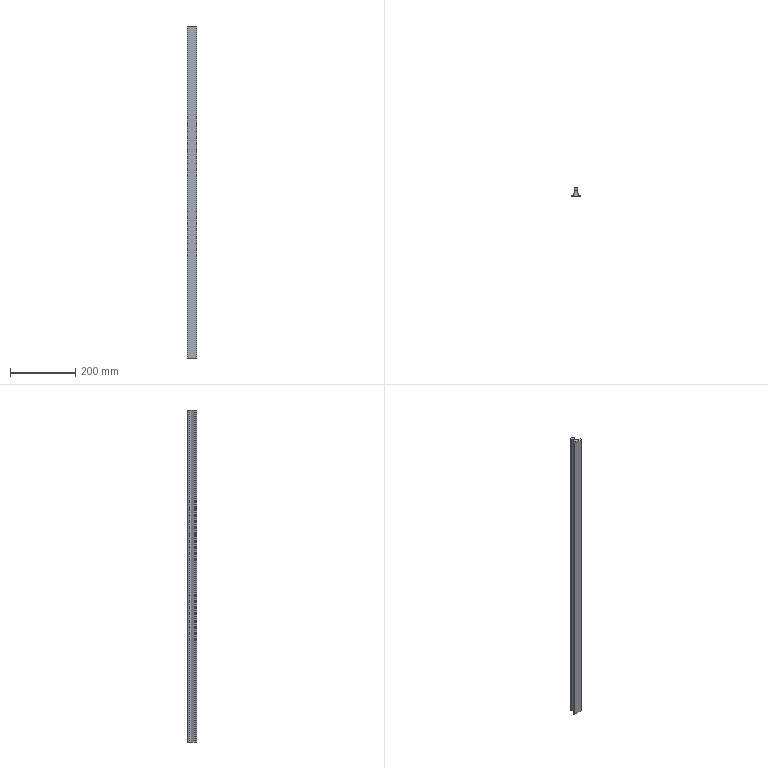Part | STEP file | SBR16S round rail_default<machined> | 2 solids | 16 faces | box 30 x 28.5 x 1020 mm | volume 387317 mm3 | plane 13 | cylinder 3 | commonest cylinder face diameters 12 x3
STEP:
#1=CARTESIAN_POINT('',(0.,0.,0.));
#2=DIRECTION('',(0.,0.,1.));
#3=DIRECTION('',(1.,0.,0.));
#4=AXIS2_PLACEMENT_3D('',#1,#2,#3);
#5=CARTESIAN_POINT('',(6.,0.,1020.));
#6=VERTEX_POINT('',#5);
#7=CARTESIAN_POINT('',(-6.,0.,1020.));
#8=VERTEX_POINT('',#7);
#9=CARTESIAN_POINT('',(0.,0.,1020.));
#10=DIRECTION('',(0.,0.,1.));
#11=DIRECTION('',(1.,0.,0.));
#12=AXIS2_PLACEMENT_3D('',#9,#10,#11);
#13=CIRCLE('',#12,6.);
#14=CARTESIAN_POINT('',(0.,0.,1020.));
#15=DIRECTION('',(0.,0.,-1.));
#16=DIRECTION('',(-1.,0.,0.));
#17=AXIS2_PLACEMENT_3D('',#14,#15,#16);
#18=CYLINDRICAL_SURFACE('',#17,6.);
#19=CARTESIAN_POINT('',(3.142,0.));
#20=DIRECTION('',(-1.,0.));
#21=VECTOR('',#20,1.);
#22=LINE('',#19,#21);
#23=(GEOMETRIC_REPRESENTATION_CONTEXT(2)PARAMETRIC_REPRESENTATION_CONTEXT()REPRESENTATION_CONTEXT('',''));
#24=DEFINITIONAL_REPRESENTATION('',(#22),#23);
#25=PCURVE('',#18,#24);
#26=CARTESIAN_POINT('',(0.,0.,1020.));
#27=DIRECTION('',(0.,0.,1.));
#28=DIRECTION('',(1.,0.,0.));
#29=AXIS2_PLACEMENT_3D('',#26,#27,#28);
#30=PLANE('',#29);
#31=CARTESIAN_POINT('',(0.,0.));
#32=DIRECTION('',(1.,0.));
#33=AXIS2_PLACEMENT_2D('',#31,#32);
#34=CIRCLE('',#33,6.);
#35=(GEOMETRIC_REPRESENTATION_CONTEXT(2)PARAMETRIC_REPRESENTATION_CONTEXT()REPRESENTATION_CONTEXT('',''));
#36=DEFINITIONAL_REPRESENTATION('',(#34),#35);
#37=PCURVE('',#30,#36);
#38=SURFACE_CURVE('',#13,(#25,#37),.PCURVE_S1.);
#39=EDGE_CURVE('',#6,#8,#38,.T.);
#40=ORIENTED_EDGE('',*,*,#39,.F.);
#41=CARTESIAN_POINT('',(6.,0.,0.));
#42=VERTEX_POINT('',#41);
#43=CARTESIAN_POINT('',(6.,0.,1020.));
#44=DIRECTION('',(0.,0.,-1.));
#45=VECTOR('',#44,1.);
#46=LINE('',#43,#45);
#47=CARTESIAN_POINT('',(3.142,0.));
#48=DIRECTION('',(0.,1.));
#49=VECTOR('',#48,1.);
#50=LINE('',#47,#49);
#51=(GEOMETRIC_REPRESENTATION_CONTEXT(2)PARAMETRIC_REPRESENTATION_CONTEXT()REPRESENTATION_CONTEXT('',''));
#52=DEFINITIONAL_REPRESENTATION('',(#50),#51);
#53=PCURVE('',#18,#52);
#54=CARTESIAN_POINT('',(0.,0.,1020.));
#55=DIRECTION('',(0.,0.,-1.));
#56=DIRECTION('',(-1.,0.,0.));
#57=AXIS2_PLACEMENT_3D('',#54,#55,#56);
#58=CYLINDRICAL_SURFACE('',#57,6.);
#59=CARTESIAN_POINT('',(3.142,0.));
#60=DIRECTION('',(0.,1.));
#61=VECTOR('',#60,1.);
#62=LINE('',#59,#61);
#63=(GEOMETRIC_REPRESENTATION_CONTEXT(2)PARAMETRIC_REPRESENTATION_CONTEXT()REPRESENTATION_CONTEXT('',''));
#64=DEFINITIONAL_REPRESENTATION('',(#62),#63);
#65=PCURVE('',#58,#64);
#66=SURFACE_CURVE('',#46,(#53,#65),.PCURVE_S1.);
#67=EDGE_CURVE('',#6,#42,#66,.T.);
#68=ORIENTED_EDGE('',*,*,#67,.T.);
#69=CARTESIAN_POINT('',(-6.,0.,0.));
#70=VERTEX_POINT('',#69);
#71=CARTESIAN_POINT('',(0.,0.,0.));
#72=DIRECTION('',(0.,0.,1.));
#73=DIRECTION('',(1.,0.,0.));
#74=AXIS2_PLACEMENT_3D('',#71,#72,#73);
#75=CIRCLE('',#74,6.);
#76=CARTESIAN_POINT('',(3.142,1020.));
#77=DIRECTION('',(-1.,0.));
#78=VECTOR('',#77,1.);
#79=LINE('',#76,#78);
#80=(GEOMETRIC_REPRESENTATION_CONTEXT(2)PARAMETRIC_REPRESENTATION_CONTEXT()REPRESENTATION_CONTEXT('',''));
#81=DEFINITIONAL_REPRESENTATION('',(#79),#80);
#82=PCURVE('',#18,#81);
#83=CARTESIAN_POINT('',(0.,0.,0.));
#84=DIRECTION('',(0.,0.,1.));
#85=DIRECTION('',(1.,0.,0.));
#86=AXIS2_PLACEMENT_3D('',#83,#84,#85);
#87=PLANE('',#86);
#88=CARTESIAN_POINT('',(0.,0.));
#89=DIRECTION('',(1.,0.));
#90=AXIS2_PLACEMENT_2D('',#88,#89);
#91=CIRCLE('',#90,6.);
#92=(GEOMETRIC_REPRESENTATION_CONTEXT(2)PARAMETRIC_REPRESENTATION_CONTEXT()REPRESENTATION_CONTEXT('',''));
#93=DEFINITIONAL_REPRESENTATION('',(#91),#92);
#94=PCURVE('',#87,#93);
#95=SURFACE_CURVE('',#75,(#82,#94),.PCURVE_S1.);
#96=EDGE_CURVE('',#42,#70,#95,.T.);
#97=ORIENTED_EDGE('',*,*,#96,.T.);
#98=CARTESIAN_POINT('',(-6.,0.,1020.));
#99=DIRECTION('',(0.,0.,-1.));
#100=VECTOR('',#99,1.);
#101=LINE('',#98,#100);
#102=CARTESIAN_POINT('',(0.,0.));
#103=DIRECTION('',(0.,1.));
#104=VECTOR('',#103,1.);
#105=LINE('',#102,#104);
#106=(GEOMETRIC_REPRESENTATION_CONTEXT(2)PARAMETRIC_REPRESENTATION_CONTEXT()REPRESENTATION_CONTEXT('',''));
#107=DEFINITIONAL_REPRESENTATION('',(#105),#106);
#108=PCURVE('',#18,#107);
#109=CARTESIAN_POINT('',(6.283,0.));
#110=DIRECTION('',(0.,1.));
#111=VECTOR('',#110,1.);
#112=LINE('',#109,#111);
#113=(GEOMETRIC_REPRESENTATION_CONTEXT(2)PARAMETRIC_REPRESENTATION_CONTEXT()REPRESENTATION_CONTEXT('',''));
#114=DEFINITIONAL_REPRESENTATION('',(#112),#113);
#115=PCURVE('',#58,#114);
#116=SURFACE_CURVE('',#101,(#108,#115),.PCURVE_S1.);
#117=EDGE_CURVE('',#8,#70,#116,.T.);
#118=ORIENTED_EDGE('',*,*,#117,.F.);
#119=EDGE_LOOP('',(#40,#68,#97,#118));
#120=FACE_BOUND('',#119,.T.);
#121=ADVANCED_FACE('',(#120),#18,.T.);
#122=ORIENTED_EDGE('',*,*,#67,.F.);
#123=CARTESIAN_POINT('',(0.,0.,1020.));
#124=DIRECTION('',(0.,0.,1.));
#125=DIRECTION('',(1.,0.,0.));
#126=AXIS2_PLACEMENT_3D('',#123,#124,#125);
#127=CIRCLE('',#126,6.);
#128=CARTESIAN_POINT('',(9.425,0.));
#129=DIRECTION('',(-1.,0.));
#130=VECTOR('',#129,1.);
#131=LINE('',#128,#130);
#132=(GEOMETRIC_REPRESENTATION_CONTEXT(2)PARAMETRIC_REPRESENTATION_CONTEXT()REPRESENTATION_CONTEXT('',''));
#133=DEFINITIONAL_REPRESENTATION('',(#131),#132);
#134=PCURVE('',#58,#133);
#135=CARTESIAN_POINT('',(0.,0.));
#136=DIRECTION('',(1.,0.));
#137=AXIS2_PLACEMENT_2D('',#135,#136);
#138=CIRCLE('',#137,6.);
#139=(GEOMETRIC_REPRESENTATION_CONTEXT(2)PARAMETRIC_REPRESENTATION_CONTEXT()REPRESENTATION_CONTEXT('',''));
#140=DEFINITIONAL_REPRESENTATION('',(#138),#139);
#141=PCURVE('',#30,#140);
#142=SURFACE_CURVE('',#127,(#134,#141),.PCURVE_S1.);
#143=EDGE_CURVE('',#8,#6,#142,.T.);
#144=ORIENTED_EDGE('',*,*,#143,.F.);
#145=ORIENTED_EDGE('',*,*,#117,.T.);
#146=CARTESIAN_POINT('',(0.,0.,0.));
#147=DIRECTION('',(0.,0.,1.));
#148=DIRECTION('',(1.,0.,0.));
#149=AXIS2_PLACEMENT_3D('',#146,#147,#148);
#150=CIRCLE('',#149,6.);
#151=CARTESIAN_POINT('',(9.425,1020.));
#152=DIRECTION('',(-1.,0.));
#153=VECTOR('',#152,1.);
#154=LINE('',#151,#153);
#155=(GEOMETRIC_REPRESENTATION_CONTEXT(2)PARAMETRIC_REPRESENTATION_CONTEXT()REPRESENTATION_CONTEXT('',''));
#156=DEFINITIONAL_REPRESENTATION('',(#154),#155);
#157=PCURVE('',#58,#156);
#158=CARTESIAN_POINT('',(0.,0.));
#159=DIRECTION('',(1.,0.));
#160=AXIS2_PLACEMENT_2D('',#158,#159);
#161=CIRCLE('',#160,6.);
#162=(GEOMETRIC_REPRESENTATION_CONTEXT(2)PARAMETRIC_REPRESENTATION_CONTEXT()REPRESENTATION_CONTEXT('',''));
#163=DEFINITIONAL_REPRESENTATION('',(#161),#162);
#164=PCURVE('',#87,#163);
#165=SURFACE_CURVE('',#150,(#157,#164),.PCURVE_S1.);
#166=EDGE_CURVE('',#70,#42,#165,.T.);
#167=ORIENTED_EDGE('',*,*,#166,.T.);
#168=EDGE_LOOP('',(#122,#144,#145,#167));
#169=FACE_BOUND('',#168,.T.);
#170=ADVANCED_FACE('',(#169),#58,.T.);
#171=ORIENTED_EDGE('',*,*,#143,.T.);
#172=ORIENTED_EDGE('',*,*,#39,.T.);
#173=EDGE_LOOP('',(#171,#172));
#174=FACE_BOUND('',#173,.T.);
#175=ADVANCED_FACE('',(#174),#30,.T.);
#176=ORIENTED_EDGE('',*,*,#166,.F.);
#177=ORIENTED_EDGE('',*,*,#96,.F.);
#178=EDGE_LOOP('',(#176,#177));
#179=FACE_BOUND('',#178,.T.);
#180=ADVANCED_FACE('',(#179),#87,.F.);
#181=CLOSED_SHELL('',(#121,#170,#175,#180));
#182=MANIFOLD_SOLID_BREP('',#181);
#183=CARTESIAN_POINT('',(2.322,-5.532,1020.));
#184=VERTEX_POINT('',#183);
#185=CARTESIAN_POINT('',(2.322,-5.532,0.));
#186=VERTEX_POINT('',#185);
#187=CARTESIAN_POINT('',(2.322,-5.532,1020.));
#188=DIRECTION('',(0.,0.,-1.));
#189=VECTOR('',#188,1.);
#190=LINE('',#187,#189);
#191=CARTESIAN_POINT('',(0.,0.,1020.));
#192=DIRECTION('',(0.,0.,-1.));
#193=DIRECTION('',(-1.,0.,0.));
#194=AXIS2_PLACEMENT_3D('',#191,#192,#193);
#195=CYLINDRICAL_SURFACE('',#194,6.);
#196=CARTESIAN_POINT('',(4.315,0.));
#197=DIRECTION('',(0.,1.));
#198=VECTOR('',#197,1.);
#199=LINE('',#196,#198);
#200=(GEOMETRIC_REPRESENTATION_CONTEXT(2)PARAMETRIC_REPRESENTATION_CONTEXT()REPRESENTATION_CONTEXT('',''));
#201=DEFINITIONAL_REPRESENTATION('',(#199),#200);
#202=PCURVE('',#195,#201);
#203=CARTESIAN_POINT('',(-0.6537,-0.3774,1020.));
#204=DIRECTION('',(-0.866,-0.5,0.));
#205=DIRECTION('',(0.5,-0.866,0.));
#206=AXIS2_PLACEMENT_3D('',#203,#204,#205);
#207=PLANE('',#206);
#208=CARTESIAN_POINT('',(5.952,0.));
#209=DIRECTION('',(0.,-1.));
#210=VECTOR('',#209,1.);
#211=LINE('',#208,#210);
#212=(GEOMETRIC_REPRESENTATION_CONTEXT(2)PARAMETRIC_REPRESENTATION_CONTEXT()REPRESENTATION_CONTEXT('',''));
#213=DEFINITIONAL_REPRESENTATION('',(#211),#212);
#214=PCURVE('',#207,#213);
#215=SURFACE_CURVE('',#190,(#202,#214),.PCURVE_S1.);
#216=EDGE_CURVE('',#184,#186,#215,.T.);
#217=ORIENTED_EDGE('',*,*,#216,.F.);
#218=CARTESIAN_POINT('',(-2.322,-5.532,1020.));
#219=VERTEX_POINT('',#218);
#220=CARTESIAN_POINT('',(0.,0.,1020.));
#221=DIRECTION('',(0.,0.,1.));
#222=DIRECTION('',(1.,0.,0.));
#223=AXIS2_PLACEMENT_3D('',#220,#221,#222);
#224=CIRCLE('',#223,6.);
#225=CARTESIAN_POINT('',(9.425,0.));
#226=DIRECTION('',(-1.,0.));
#227=VECTOR('',#226,1.);
#228=LINE('',#225,#227);
#229=(GEOMETRIC_REPRESENTATION_CONTEXT(2)PARAMETRIC_REPRESENTATION_CONTEXT()REPRESENTATION_CONTEXT('',''));
#230=DEFINITIONAL_REPRESENTATION('',(#228),#229);
#231=PCURVE('',#195,#230);
#232=CARTESIAN_POINT('',(0.,0.,1020.));
#233=DIRECTION('',(0.,0.,1.));
#234=DIRECTION('',(1.,0.,0.));
#235=AXIS2_PLACEMENT_3D('',#232,#233,#234);
#236=PLANE('',#235);
#237=CARTESIAN_POINT('',(0.,0.));
#238=DIRECTION('',(1.,0.));
#239=AXIS2_PLACEMENT_2D('',#237,#238);
#240=CIRCLE('',#239,6.);
#241=(GEOMETRIC_REPRESENTATION_CONTEXT(2)PARAMETRIC_REPRESENTATION_CONTEXT()REPRESENTATION_CONTEXT('',''));
#242=DEFINITIONAL_REPRESENTATION('',(#240),#241);
#243=PCURVE('',#236,#242);
#244=SURFACE_CURVE('',#224,(#231,#243),.PCURVE_S1.);
#245=EDGE_CURVE('',#219,#184,#244,.T.);
#246=ORIENTED_EDGE('',*,*,#245,.F.);
#247=CARTESIAN_POINT('',(-2.322,-5.532,0.));
#248=VERTEX_POINT('',#247);
#249=CARTESIAN_POINT('',(-2.322,-5.532,1020.));
#250=DIRECTION('',(0.,0.,-1.));
#251=VECTOR('',#250,1.);
#252=LINE('',#249,#251);
#253=CARTESIAN_POINT('',(5.11,0.));
#254=DIRECTION('',(0.,1.));
#255=VECTOR('',#254,1.);
#256=LINE('',#253,#255);
#257=(GEOMETRIC_REPRESENTATION_CONTEXT(2)PARAMETRIC_REPRESENTATION_CONTEXT()REPRESENTATION_CONTEXT('',''));
#258=DEFINITIONAL_REPRESENTATION('',(#256),#257);
#259=PCURVE('',#195,#258);
#260=CARTESIAN_POINT('',(0.6537,-0.3774,1020.));
#261=DIRECTION('',(-0.866,0.5,0.));
#262=DIRECTION('',(-0.5,-0.866,0.));
#263=AXIS2_PLACEMENT_3D('',#260,#261,#262);
#264=PLANE('',#263);
#265=CARTESIAN_POINT('',(5.952,0.));
#266=DIRECTION('',(0.,-1.));
#267=VECTOR('',#266,1.);
#268=LINE('',#265,#267);
#269=(GEOMETRIC_REPRESENTATION_CONTEXT(2)PARAMETRIC_REPRESENTATION_CONTEXT()REPRESENTATION_CONTEXT('',''));
#270=DEFINITIONAL_REPRESENTATION('',(#268),#269);
#271=PCURVE('',#264,#270);
#272=SURFACE_CURVE('',#252,(#259,#271),.PCURVE_S1.);
#273=EDGE_CURVE('',#219,#248,#272,.T.);
#274=ORIENTED_EDGE('',*,*,#273,.T.);
#275=CARTESIAN_POINT('',(0.,0.,0.));
#276=DIRECTION('',(0.,0.,1.));
#277=DIRECTION('',(1.,0.,0.));
#278=AXIS2_PLACEMENT_3D('',#275,#276,#277);
#279=CIRCLE('',#278,6.);
#280=CARTESIAN_POINT('',(9.425,1020.));
#281=DIRECTION('',(-1.,0.));
#282=VECTOR('',#281,1.);
#283=LINE('',#280,#282);
#284=(GEOMETRIC_REPRESENTATION_CONTEXT(2)PARAMETRIC_REPRESENTATION_CONTEXT()REPRESENTATION_CONTEXT('',''));
#285=DEFINITIONAL_REPRESENTATION('',(#283),#284);
#286=PCURVE('',#195,#285);
#287=CARTESIAN_POINT('',(0.,0.,0.));
#288=DIRECTION('',(0.,0.,1.));
#289=DIRECTION('',(1.,0.,0.));
#290=AXIS2_PLACEMENT_3D('',#287,#288,#289);
#291=PLANE('',#290);
#292=CARTESIAN_POINT('',(0.,0.));
#293=DIRECTION('',(1.,0.));
#294=AXIS2_PLACEMENT_2D('',#292,#293);
#295=CIRCLE('',#294,6.);
#296=(GEOMETRIC_REPRESENTATION_CONTEXT(2)PARAMETRIC_REPRESENTATION_CONTEXT()REPRESENTATION_CONTEXT('',''));
#297=DEFINITIONAL_REPRESENTATION('',(#295),#296);
#298=PCURVE('',#291,#297);
#299=SURFACE_CURVE('',#279,(#286,#298),.PCURVE_S1.);
#300=EDGE_CURVE('',#248,#186,#299,.T.);
#301=ORIENTED_EDGE('',*,*,#300,.T.);
#302=EDGE_LOOP('',(#217,#246,#274,#301));
#303=FACE_BOUND('',#302,.F.);
#304=ADVANCED_FACE('',(#303),#195,.F.);
#305=CARTESIAN_POINT('',(-7.5,-14.5,0.));
#306=VERTEX_POINT('',#305);
#307=CARTESIAN_POINT('',(0.6537,-0.3774,0.));
#308=DIRECTION('',(0.5,0.866,0.));
#309=VECTOR('',#308,1.);
#310=LINE('',#307,#309);
#311=CARTESIAN_POINT('',(0.,-1020.));
#312=DIRECTION('',(-1.,0.));
#313=VECTOR('',#312,1.);
#314=LINE('',#311,#313);
#315=(GEOMETRIC_REPRESENTATION_CONTEXT(2)PARAMETRIC_REPRESENTATION_CONTEXT()REPRESENTATION_CONTEXT('',''));
#316=DEFINITIONAL_REPRESENTATION('',(#314),#315);
#317=PCURVE('',#264,#316);
#318=CARTESIAN_POINT('',(0.6537,-0.3774));
#319=DIRECTION('',(0.5,0.866));
#320=VECTOR('',#319,1.);
#321=LINE('',#318,#320);
#322=(GEOMETRIC_REPRESENTATION_CONTEXT(2)PARAMETRIC_REPRESENTATION_CONTEXT()REPRESENTATION_CONTEXT('',''));
#323=DEFINITIONAL_REPRESENTATION('',(#321),#322);
#324=PCURVE('',#291,#323);
#325=SURFACE_CURVE('',#310,(#317,#324),.PCURVE_S1.);
#326=EDGE_CURVE('',#306,#248,#325,.T.);
#327=ORIENTED_EDGE('',*,*,#326,.F.);
#328=CARTESIAN_POINT('',(-7.5,-14.5,1020.));
#329=VERTEX_POINT('',#328);
#330=CARTESIAN_POINT('',(-7.5,-14.5,1020.));
#331=DIRECTION('',(0.,0.,-1.));
#332=VECTOR('',#331,1.);
#333=LINE('',#330,#332);
#334=CARTESIAN_POINT('',(16.307,0.));
#335=DIRECTION('',(0.,-1.));
#336=VECTOR('',#335,1.);
#337=LINE('',#334,#336);
#338=(GEOMETRIC_REPRESENTATION_CONTEXT(2)PARAMETRIC_REPRESENTATION_CONTEXT()REPRESENTATION_CONTEXT('',''));
#339=DEFINITIONAL_REPRESENTATION('',(#337),#338);
#340=PCURVE('',#264,#339);
#341=CARTESIAN_POINT('',(-7.5,0.,1020.));
#342=DIRECTION('',(-1.,0.,0.));
#343=DIRECTION('',(0.,0.,1.));
#344=AXIS2_PLACEMENT_3D('',#341,#342,#343);
#345=PLANE('',#344);
#346=CARTESIAN_POINT('',(0.,-14.5));
#347=DIRECTION('',(-1.,0.));
#348=VECTOR('',#347,1.);
#349=LINE('',#346,#348);
#350=(GEOMETRIC_REPRESENTATION_CONTEXT(2)PARAMETRIC_REPRESENTATION_CONTEXT()REPRESENTATION_CONTEXT('',''));
#351=DEFINITIONAL_REPRESENTATION('',(#349),#350);
#352=PCURVE('',#345,#351);
#353=SURFACE_CURVE('',#333,(#340,#352),.PCURVE_S1.);
#354=EDGE_CURVE('',#329,#306,#353,.T.);
#355=ORIENTED_EDGE('',*,*,#354,.F.);
#356=CARTESIAN_POINT('',(0.6537,-0.3774,1020.));
#357=DIRECTION('',(0.5,0.866,0.));
#358=VECTOR('',#357,1.);
#359=LINE('',#356,#358);
#360=CARTESIAN_POINT('',(0.,0.));
#361=DIRECTION('',(-1.,0.));
#362=VECTOR('',#361,1.);
#363=LINE('',#360,#362);
#364=(GEOMETRIC_REPRESENTATION_CONTEXT(2)PARAMETRIC_REPRESENTATION_CONTEXT()REPRESENTATION_CONTEXT('',''));
#365=DEFINITIONAL_REPRESENTATION('',(#363),#364);
#366=PCURVE('',#264,#365);
#367=CARTESIAN_POINT('',(0.6537,-0.3774));
#368=DIRECTION('',(0.5,0.866));
#369=VECTOR('',#368,1.);
#370=LINE('',#367,#369);
#371=(GEOMETRIC_REPRESENTATION_CONTEXT(2)PARAMETRIC_REPRESENTATION_CONTEXT()REPRESENTATION_CONTEXT('',''));
#372=DEFINITIONAL_REPRESENTATION('',(#370),#371);
#373=PCURVE('',#236,#372);
#374=SURFACE_CURVE('',#359,(#366,#373),.PCURVE_S1.);
#375=EDGE_CURVE('',#329,#219,#374,.T.);
#376=ORIENTED_EDGE('',*,*,#375,.T.);
#377=ORIENTED_EDGE('',*,*,#273,.T.);
#378=EDGE_LOOP('',(#327,#355,#376,#377));
#379=FACE_BOUND('',#378,.T.);
#380=ADVANCED_FACE('',(#379),#264,.T.);
#381=CARTESIAN_POINT('',(-7.5,-18.5,0.));
#382=VERTEX_POINT('',#381);
#383=CARTESIAN_POINT('',(-7.5,0.,0.));
#384=DIRECTION('',(0.,1.,0.));
#385=VECTOR('',#384,1.);
#386=LINE('',#383,#385);
#387=CARTESIAN_POINT('',(-1020.,0.));
#388=DIRECTION('',(0.,1.));
#389=VECTOR('',#388,1.);
#390=LINE('',#387,#389);
#391=(GEOMETRIC_REPRESENTATION_CONTEXT(2)PARAMETRIC_REPRESENTATION_CONTEXT()REPRESENTATION_CONTEXT('',''));
#392=DEFINITIONAL_REPRESENTATION('',(#390),#391);
#393=PCURVE('',#345,#392);
#394=CARTESIAN_POINT('',(-7.5,0.));
#395=DIRECTION('',(0.,1.));
#396=VECTOR('',#395,1.);
#397=LINE('',#394,#396);
#398=(GEOMETRIC_REPRESENTATION_CONTEXT(2)PARAMETRIC_REPRESENTATION_CONTEXT()REPRESENTATION_CONTEXT('',''));
#399=DEFINITIONAL_REPRESENTATION('',(#397),#398);
#400=PCURVE('',#291,#399);
#401=SURFACE_CURVE('',#386,(#393,#400),.PCURVE_S1.);
#402=EDGE_CURVE('',#382,#306,#401,.T.);
#403=ORIENTED_EDGE('',*,*,#402,.F.);
#404=CARTESIAN_POINT('',(-7.5,-18.5,1020.));
#405=VERTEX_POINT('',#404);
#406=CARTESIAN_POINT('',(-7.5,-18.5,1020.));
#407=DIRECTION('',(0.,0.,-1.));
#408=VECTOR('',#407,1.);
#409=LINE('',#406,#408);
#410=CARTESIAN_POINT('',(0.,-18.5));
#411=DIRECTION('',(-1.,0.));
#412=VECTOR('',#411,1.);
#413=LINE('',#410,#412);
#414=(GEOMETRIC_REPRESENTATION_CONTEXT(2)PARAMETRIC_REPRESENTATION_CONTEXT()REPRESENTATION_CONTEXT('',''));
#415=DEFINITIONAL_REPRESENTATION('',(#413),#414);
#416=PCURVE('',#345,#415);
#417=CARTESIAN_POINT('',(0.,-18.5,1020.));
#418=DIRECTION('',(0.,1.,0.));
#419=DIRECTION('',(0.,0.,1.));
#420=AXIS2_PLACEMENT_3D('',#417,#418,#419);
#421=PLANE('',#420);
#422=CARTESIAN_POINT('',(0.,-7.5));
#423=DIRECTION('',(-1.,0.));
#424=VECTOR('',#423,1.);
#425=LINE('',#422,#424);
#426=(GEOMETRIC_REPRESENTATION_CONTEXT(2)PARAMETRIC_REPRESENTATION_CONTEXT()REPRESENTATION_CONTEXT('',''));
#427=DEFINITIONAL_REPRESENTATION('',(#425),#426);
#428=PCURVE('',#421,#427);
#429=SURFACE_CURVE('',#409,(#416,#428),.PCURVE_S1.);
#430=EDGE_CURVE('',#405,#382,#429,.T.);
#431=ORIENTED_EDGE('',*,*,#430,.F.);
#432=CARTESIAN_POINT('',(-7.5,0.,1020.));
#433=DIRECTION('',(0.,1.,0.));
#434=VECTOR('',#433,1.);
#435=LINE('',#432,#434);
#436=CARTESIAN_POINT('',(0.,0.));
#437=DIRECTION('',(0.,1.));
#438=VECTOR('',#437,1.);
#439=LINE('',#436,#438);
#440=(GEOMETRIC_REPRESENTATION_CONTEXT(2)PARAMETRIC_REPRESENTATION_CONTEXT()REPRESENTATION_CONTEXT('',''));
#441=DEFINITIONAL_REPRESENTATION('',(#439),#440);
#442=PCURVE('',#345,#441);
#443=CARTESIAN_POINT('',(-7.5,0.));
#444=DIRECTION('',(0.,1.));
#445=VECTOR('',#444,1.);
#446=LINE('',#443,#445);
#447=(GEOMETRIC_REPRESENTATION_CONTEXT(2)PARAMETRIC_REPRESENTATION_CONTEXT()REPRESENTATION_CONTEXT('',''));
#448=DEFINITIONAL_REPRESENTATION('',(#446),#447);
#449=PCURVE('',#236,#448);
#450=SURFACE_CURVE('',#435,(#442,#449),.PCURVE_S1.);
#451=EDGE_CURVE('',#405,#329,#450,.T.);
#452=ORIENTED_EDGE('',*,*,#451,.T.);
#453=ORIENTED_EDGE('',*,*,#354,.T.);
#454=EDGE_LOOP('',(#403,#431,#452,#453));
#455=FACE_BOUND('',#454,.T.);
#456=ADVANCED_FACE('',(#455),#345,.T.);
#457=CARTESIAN_POINT('',(-15.,-18.5,0.));
#458=VERTEX_POINT('',#457);
#459=CARTESIAN_POINT('',(0.,-18.5,0.));
#460=DIRECTION('',(1.,0.,0.));
#461=VECTOR('',#460,1.);
#462=LINE('',#459,#461);
#463=CARTESIAN_POINT('',(-1020.,0.));
#464=DIRECTION('',(0.,1.));
#465=VECTOR('',#464,1.);
#466=LINE('',#463,#465);
#467=(GEOMETRIC_REPRESENTATION_CONTEXT(2)PARAMETRIC_REPRESENTATION_CONTEXT()REPRESENTATION_CONTEXT('',''));
#468=DEFINITIONAL_REPRESENTATION('',(#466),#467);
#469=PCURVE('',#421,#468);
#470=CARTESIAN_POINT('',(0.,-18.5));
#471=DIRECTION('',(1.,0.));
#472=VECTOR('',#471,1.);
#473=LINE('',#470,#472);
#474=(GEOMETRIC_REPRESENTATION_CONTEXT(2)PARAMETRIC_REPRESENTATION_CONTEXT()REPRESENTATION_CONTEXT('',''));
#475=DEFINITIONAL_REPRESENTATION('',(#473),#474);
#476=PCURVE('',#291,#475);
#477=SURFACE_CURVE('',#462,(#469,#476),.PCURVE_S1.);
#478=EDGE_CURVE('',#458,#382,#477,.T.);
#479=ORIENTED_EDGE('',*,*,#478,.F.);
#480=CARTESIAN_POINT('',(-15.,-18.5,1020.));
#481=VERTEX_POINT('',#480);
#482=CARTESIAN_POINT('',(-15.,-18.5,1020.));
#483=DIRECTION('',(0.,0.,-1.));
#484=VECTOR('',#483,1.);
#485=LINE('',#482,#484);
#486=CARTESIAN_POINT('',(0.,-15.));
#487=DIRECTION('',(-1.,0.));
#488=VECTOR('',#487,1.);
#489=LINE('',#486,#488);
#490=(GEOMETRIC_REPRESENTATION_CONTEXT(2)PARAMETRIC_REPRESENTATION_CONTEXT()REPRESENTATION_CONTEXT('',''));
#491=DEFINITIONAL_REPRESENTATION('',(#489),#490);
#492=PCURVE('',#421,#491);
#493=CARTESIAN_POINT('',(-15.,0.,1020.));
#494=DIRECTION('',(-1.,0.,0.));
#495=DIRECTION('',(0.,0.,1.));
#496=AXIS2_PLACEMENT_3D('',#493,#494,#495);
#497=PLANE('',#496);
#498=CARTESIAN_POINT('',(0.,-18.5));
#499=DIRECTION('',(-1.,0.));
#500=VECTOR('',#499,1.);
#501=LINE('',#498,#500);
#502=(GEOMETRIC_REPRESENTATION_CONTEXT(2)PARAMETRIC_REPRESENTATION_CONTEXT()REPRESENTATION_CONTEXT('',''));
#503=DEFINITIONAL_REPRESENTATION('',(#501),#502);
#504=PCURVE('',#497,#503);
#505=SURFACE_CURVE('',#485,(#492,#504),.PCURVE_S1.);
#506=EDGE_CURVE('',#481,#458,#505,.T.);
#507=ORIENTED_EDGE('',*,*,#506,.F.);
#508=CARTESIAN_POINT('',(0.,-18.5,1020.));
#509=DIRECTION('',(1.,0.,0.));
#510=VECTOR('',#509,1.);
#511=LINE('',#508,#510);
#512=CARTESIAN_POINT('',(0.,0.));
#513=DIRECTION('',(0.,1.));
#514=VECTOR('',#513,1.);
#515=LINE('',#512,#514);
#516=(GEOMETRIC_REPRESENTATION_CONTEXT(2)PARAMETRIC_REPRESENTATION_CONTEXT()REPRESENTATION_CONTEXT('',''));
#517=DEFINITIONAL_REPRESENTATION('',(#515),#516);
#518=PCURVE('',#421,#517);
#519=CARTESIAN_POINT('',(0.,-18.5));
#520=DIRECTION('',(1.,0.));
#521=VECTOR('',#520,1.);
#522=LINE('',#519,#521);
#523=(GEOMETRIC_REPRESENTATION_CONTEXT(2)PARAMETRIC_REPRESENTATION_CONTEXT()REPRESENTATION_CONTEXT('',''));
#524=DEFINITIONAL_REPRESENTATION('',(#522),#523);
#525=PCURVE('',#236,#524);
#526=SURFACE_CURVE('',#511,(#518,#525),.PCURVE_S1.);
#527=EDGE_CURVE('',#481,#405,#526,.T.);
#528=ORIENTED_EDGE('',*,*,#527,.T.);
#529=ORIENTED_EDGE('',*,*,#430,.T.);
#530=EDGE_LOOP('',(#479,#507,#528,#529));
#531=FACE_BOUND('',#530,.T.);
#532=ADVANCED_FACE('',(#531),#421,.T.);
#533=CARTESIAN_POINT('',(-15.,-22.5,0.));
#534=VERTEX_POINT('',#533);
#535=CARTESIAN_POINT('',(-15.,0.,0.));
#536=DIRECTION('',(0.,1.,0.));
#537=VECTOR('',#536,1.);
#538=LINE('',#535,#537);
#539=CARTESIAN_POINT('',(-1020.,0.));
#540=DIRECTION('',(0.,1.));
#541=VECTOR('',#540,1.);
#542=LINE('',#539,#541);
#543=(GEOMETRIC_REPRESENTATION_CONTEXT(2)PARAMETRIC_REPRESENTATION_CONTEXT()REPRESENTATION_CONTEXT('',''));
#544=DEFINITIONAL_REPRESENTATION('',(#542),#543);
#545=PCURVE('',#497,#544);
#546=CARTESIAN_POINT('',(-15.,0.));
#547=DIRECTION('',(0.,1.));
#548=VECTOR('',#547,1.);
#549=LINE('',#546,#548);
#550=(GEOMETRIC_REPRESENTATION_CONTEXT(2)PARAMETRIC_REPRESENTATION_CONTEXT()REPRESENTATION_CONTEXT('',''));
#551=DEFINITIONAL_REPRESENTATION('',(#549),#550);
#552=PCURVE('',#291,#551);
#553=SURFACE_CURVE('',#538,(#545,#552),.PCURVE_S1.);
#554=EDGE_CURVE('',#534,#458,#553,.T.);
#555=ORIENTED_EDGE('',*,*,#554,.F.);
#556=CARTESIAN_POINT('',(-15.,-22.5,1020.));
#557=VERTEX_POINT('',#556);
#558=CARTESIAN_POINT('',(-15.,-22.5,1020.));
#559=DIRECTION('',(0.,0.,-1.));
#560=VECTOR('',#559,1.);
#561=LINE('',#558,#560);
#562=CARTESIAN_POINT('',(0.,-22.5));
#563=DIRECTION('',(-1.,0.));
#564=VECTOR('',#563,1.);
#565=LINE('',#562,#564);
#566=(GEOMETRIC_REPRESENTATION_CONTEXT(2)PARAMETRIC_REPRESENTATION_CONTEXT()REPRESENTATION_CONTEXT('',''));
#567=DEFINITIONAL_REPRESENTATION('',(#565),#566);
#568=PCURVE('',#497,#567);
#569=CARTESIAN_POINT('',(0.,-22.5,1020.));
#570=DIRECTION('',(0.,1.,0.));
#571=DIRECTION('',(0.,0.,1.));
#572=AXIS2_PLACEMENT_3D('',#569,#570,#571);
#573=PLANE('',#572);
#574=CARTESIAN_POINT('',(0.,-15.));
#575=DIRECTION('',(-1.,0.));
#576=VECTOR('',#575,1.);
#577=LINE('',#574,#576);
#578=(GEOMETRIC_REPRESENTATION_CONTEXT(2)PARAMETRIC_REPRESENTATION_CONTEXT()REPRESENTATION_CONTEXT('',''));
#579=DEFINITIONAL_REPRESENTATION('',(#577),#578);
#580=PCURVE('',#573,#579);
#581=SURFACE_CURVE('',#561,(#568,#580),.PCURVE_S1.);
#582=EDGE_CURVE('',#557,#534,#581,.T.);
#583=ORIENTED_EDGE('',*,*,#582,.F.);
#584=CARTESIAN_POINT('',(-15.,0.,1020.));
#585=DIRECTION('',(0.,1.,0.));
#586=VECTOR('',#585,1.);
#587=LINE('',#584,#586);
#588=CARTESIAN_POINT('',(0.,0.));
#589=DIRECTION('',(0.,1.));
#590=VECTOR('',#589,1.);
#591=LINE('',#588,#590);
#592=(GEOMETRIC_REPRESENTATION_CONTEXT(2)PARAMETRIC_REPRESENTATION_CONTEXT()REPRESENTATION_CONTEXT('',''));
#593=DEFINITIONAL_REPRESENTATION('',(#591),#592);
#594=PCURVE('',#497,#593);
#595=CARTESIAN_POINT('',(-15.,0.));
#596=DIRECTION('',(0.,1.));
#597=VECTOR('',#596,1.);
#598=LINE('',#595,#597);
#599=(GEOMETRIC_REPRESENTATION_CONTEXT(2)PARAMETRIC_REPRESENTATION_CONTEXT()REPRESENTATION_CONTEXT('',''));
#600=DEFINITIONAL_REPRESENTATION('',(#598),#599);
#601=PCURVE('',#236,#600);
#602=SURFACE_CURVE('',#587,(#594,#601),.PCURVE_S1.);
#603=EDGE_CURVE('',#557,#481,#602,.T.);
#604=ORIENTED_EDGE('',*,*,#603,.T.);
#605=ORIENTED_EDGE('',*,*,#506,.T.);
#606=EDGE_LOOP('',(#555,#583,#604,#605));
#607=FACE_BOUND('',#606,.T.);
#608=ADVANCED_FACE('',(#607),#497,.T.);
#609=CARTESIAN_POINT('',(15.,-22.5,0.));
#610=VERTEX_POINT('',#609);
#611=CARTESIAN_POINT('',(0.,-22.5,0.));
#612=DIRECTION('',(1.,0.,0.));
#613=VECTOR('',#612,1.);
#614=LINE('',#611,#613);
#615=CARTESIAN_POINT('',(-1020.,0.));
#616=DIRECTION('',(0.,1.));
#617=VECTOR('',#616,1.);
#618=LINE('',#615,#617);
#619=(GEOMETRIC_REPRESENTATION_CONTEXT(2)PARAMETRIC_REPRESENTATION_CONTEXT()REPRESENTATION_CONTEXT('',''));
#620=DEFINITIONAL_REPRESENTATION('',(#618),#619);
#621=PCURVE('',#573,#620);
#622=CARTESIAN_POINT('',(0.,-22.5));
#623=DIRECTION('',(1.,0.));
#624=VECTOR('',#623,1.);
#625=LINE('',#622,#624);
#626=(GEOMETRIC_REPRESENTATION_CONTEXT(2)PARAMETRIC_REPRESENTATION_CONTEXT()REPRESENTATION_CONTEXT('',''));
#627=DEFINITIONAL_REPRESENTATION('',(#625),#626);
#628=PCURVE('',#291,#627);
#629=SURFACE_CURVE('',#614,(#621,#628),.PCURVE_S1.);
#630=EDGE_CURVE('',#534,#610,#629,.T.);
#631=ORIENTED_EDGE('',*,*,#630,.T.);
#632=CARTESIAN_POINT('',(15.,-22.5,1020.));
#633=VERTEX_POINT('',#632);
#634=CARTESIAN_POINT('',(15.,-22.5,1020.));
#635=DIRECTION('',(0.,0.,-1.));
#636=VECTOR('',#635,1.);
#637=LINE('',#634,#636);
#638=CARTESIAN_POINT('',(0.,15.));
#639=DIRECTION('',(-1.,0.));
#640=VECTOR('',#639,1.);
#641=LINE('',#638,#640);
#642=(GEOMETRIC_REPRESENTATION_CONTEXT(2)PARAMETRIC_REPRESENTATION_CONTEXT()REPRESENTATION_CONTEXT('',''));
#643=DEFINITIONAL_REPRESENTATION('',(#641),#642);
#644=PCURVE('',#573,#643);
#645=CARTESIAN_POINT('',(15.,0.,1020.));
#646=DIRECTION('',(1.,0.,0.));
#647=DIRECTION('',(0.,0.,-1.));
#648=AXIS2_PLACEMENT_3D('',#645,#646,#647);
#649=PLANE('',#648);
#650=CARTESIAN_POINT('',(0.,-22.5));
#651=DIRECTION('',(1.,0.));
#652=VECTOR('',#651,1.);
#653=LINE('',#650,#652);
#654=(GEOMETRIC_REPRESENTATION_CONTEXT(2)PARAMETRIC_REPRESENTATION_CONTEXT()REPRESENTATION_CONTEXT('',''));
#655=DEFINITIONAL_REPRESENTATION('',(#653),#654);
#656=PCURVE('',#649,#655);
#657=SURFACE_CURVE('',#637,(#644,#656),.PCURVE_S1.);
#658=EDGE_CURVE('',#633,#610,#657,.T.);
#659=ORIENTED_EDGE('',*,*,#658,.F.);
#660=CARTESIAN_POINT('',(0.,-22.5,1020.));
#661=DIRECTION('',(1.,0.,0.));
#662=VECTOR('',#661,1.);
#663=LINE('',#660,#662);
#664=CARTESIAN_POINT('',(0.,0.));
#665=DIRECTION('',(0.,1.));
#666=VECTOR('',#665,1.);
#667=LINE('',#664,#666);
#668=(GEOMETRIC_REPRESENTATION_CONTEXT(2)PARAMETRIC_REPRESENTATION_CONTEXT()REPRESENTATION_CONTEXT('',''));
#669=DEFINITIONAL_REPRESENTATION('',(#667),#668);
#670=PCURVE('',#573,#669);
#671=CARTESIAN_POINT('',(0.,-22.5));
#672=DIRECTION('',(1.,0.));
#673=VECTOR('',#672,1.);
#674=LINE('',#671,#673);
#675=(GEOMETRIC_REPRESENTATION_CONTEXT(2)PARAMETRIC_REPRESENTATION_CONTEXT()REPRESENTATION_CONTEXT('',''));
#676=DEFINITIONAL_REPRESENTATION('',(#674),#675);
#677=PCURVE('',#236,#676);
#678=SURFACE_CURVE('',#663,(#670,#677),.PCURVE_S1.);
#679=EDGE_CURVE('',#557,#633,#678,.T.);
#680=ORIENTED_EDGE('',*,*,#679,.F.);
#681=ORIENTED_EDGE('',*,*,#582,.T.);
#682=EDGE_LOOP('',(#631,#659,#680,#681));
#683=FACE_BOUND('',#682,.T.);
#684=ADVANCED_FACE('',(#683),#573,.F.);
#685=CARTESIAN_POINT('',(15.,-18.5,0.));
#686=VERTEX_POINT('',#685);
#687=CARTESIAN_POINT('',(15.,0.,0.));
#688=DIRECTION('',(0.,-1.,0.));
#689=VECTOR('',#688,1.);
#690=LINE('',#687,#689);
#691=CARTESIAN_POINT('',(1020.,0.));
#692=DIRECTION('',(0.,-1.));
#693=VECTOR('',#692,1.);
#694=LINE('',#691,#693);
#695=(GEOMETRIC_REPRESENTATION_CONTEXT(2)PARAMETRIC_REPRESENTATION_CONTEXT()REPRESENTATION_CONTEXT('',''));
#696=DEFINITIONAL_REPRESENTATION('',(#694),#695);
#697=PCURVE('',#649,#696);
#698=CARTESIAN_POINT('',(15.,0.));
#699=DIRECTION('',(0.,-1.));
#700=VECTOR('',#699,1.);
#701=LINE('',#698,#700);
#702=(GEOMETRIC_REPRESENTATION_CONTEXT(2)PARAMETRIC_REPRESENTATION_CONTEXT()REPRESENTATION_CONTEXT('',''));
#703=DEFINITIONAL_REPRESENTATION('',(#701),#702);
#704=PCURVE('',#291,#703);
#705=SURFACE_CURVE('',#690,(#697,#704),.PCURVE_S1.);
#706=EDGE_CURVE('',#686,#610,#705,.T.);
#707=ORIENTED_EDGE('',*,*,#706,.F.);
#708=CARTESIAN_POINT('',(15.,-18.5,1020.));
#709=VERTEX_POINT('',#708);
#710=CARTESIAN_POINT('',(15.,-18.5,1020.));
#711=DIRECTION('',(0.,0.,-1.));
#712=VECTOR('',#711,1.);
#713=LINE('',#710,#712);
#714=CARTESIAN_POINT('',(0.,-18.5));
#715=DIRECTION('',(1.,0.));
#716=VECTOR('',#715,1.);
#717=LINE('',#714,#716);
#718=(GEOMETRIC_REPRESENTATION_CONTEXT(2)PARAMETRIC_REPRESENTATION_CONTEXT()REPRESENTATION_CONTEXT('',''));
#719=DEFINITIONAL_REPRESENTATION('',(#717),#718);
#720=PCURVE('',#649,#719);
#721=CARTESIAN_POINT('',(0.,-18.5,1020.));
#722=DIRECTION('',(0.,-1.,0.));
#723=DIRECTION('',(0.,0.,-1.));
#724=AXIS2_PLACEMENT_3D('',#721,#722,#723);
#725=PLANE('',#724);
#726=CARTESIAN_POINT('',(0.,15.));
#727=DIRECTION('',(1.,0.));
#728=VECTOR('',#727,1.);
#729=LINE('',#726,#728);
#730=(GEOMETRIC_REPRESENTATION_CONTEXT(2)PARAMETRIC_REPRESENTATION_CONTEXT()REPRESENTATION_CONTEXT('',''));
#731=DEFINITIONAL_REPRESENTATION('',(#729),#730);
#732=PCURVE('',#725,#731);
#733=SURFACE_CURVE('',#713,(#720,#732),.PCURVE_S1.);
#734=EDGE_CURVE('',#709,#686,#733,.T.);
#735=ORIENTED_EDGE('',*,*,#734,.F.);
#736=CARTESIAN_POINT('',(15.,0.,1020.));
#737=DIRECTION('',(0.,-1.,0.));
#738=VECTOR('',#737,1.);
#739=LINE('',#736,#738);
#740=CARTESIAN_POINT('',(0.,0.));
#741=DIRECTION('',(0.,-1.));
#742=VECTOR('',#741,1.);
#743=LINE('',#740,#742);
#744=(GEOMETRIC_REPRESENTATION_CONTEXT(2)PARAMETRIC_REPRESENTATION_CONTEXT()REPRESENTATION_CONTEXT('',''));
#745=DEFINITIONAL_REPRESENTATION('',(#743),#744);
#746=PCURVE('',#649,#745);
#747=CARTESIAN_POINT('',(15.,0.));
#748=DIRECTION('',(0.,-1.));
#749=VECTOR('',#748,1.);
#750=LINE('',#747,#749);
#751=(GEOMETRIC_REPRESENTATION_CONTEXT(2)PARAMETRIC_REPRESENTATION_CONTEXT()REPRESENTATION_CONTEXT('',''));
#752=DEFINITIONAL_REPRESENTATION('',(#750),#751);
#753=PCURVE('',#236,#752);
#754=SURFACE_CURVE('',#739,(#746,#753),.PCURVE_S1.);
#755=EDGE_CURVE('',#709,#633,#754,.T.);
#756=ORIENTED_EDGE('',*,*,#755,.T.);
#757=ORIENTED_EDGE('',*,*,#658,.T.);
#758=EDGE_LOOP('',(#707,#735,#756,#757));
#759=FACE_BOUND('',#758,.T.);
#760=ADVANCED_FACE('',(#759),#649,.T.);
#761=CARTESIAN_POINT('',(7.5,-18.5,0.));
#762=VERTEX_POINT('',#761);
#763=CARTESIAN_POINT('',(0.,-18.5,0.));
#764=DIRECTION('',(-1.,0.,0.));
#765=VECTOR('',#764,1.);
#766=LINE('',#763,#765);
#767=CARTESIAN_POINT('',(1020.,0.));
#768=DIRECTION('',(0.,-1.));
#769=VECTOR('',#768,1.);
#770=LINE('',#767,#769);
#771=(GEOMETRIC_REPRESENTATION_CONTEXT(2)PARAMETRIC_REPRESENTATION_CONTEXT()REPRESENTATION_CONTEXT('',''));
#772=DEFINITIONAL_REPRESENTATION('',(#770),#771);
#773=PCURVE('',#725,#772);
#774=CARTESIAN_POINT('',(0.,-18.5));
#775=DIRECTION('',(-1.,0.));
#776=VECTOR('',#775,1.);
#777=LINE('',#774,#776);
#778=(GEOMETRIC_REPRESENTATION_CONTEXT(2)PARAMETRIC_REPRESENTATION_CONTEXT()REPRESENTATION_CONTEXT('',''));
#779=DEFINITIONAL_REPRESENTATION('',(#777),#778);
#780=PCURVE('',#291,#779);
#781=SURFACE_CURVE('',#766,(#773,#780),.PCURVE_S1.);
#782=EDGE_CURVE('',#686,#762,#781,.T.);
#783=ORIENTED_EDGE('',*,*,#782,.T.);
#784=CARTESIAN_POINT('',(7.5,-18.5,1020.));
#785=VERTEX_POINT('',#784);
#786=CARTESIAN_POINT('',(7.5,-18.5,1020.));
#787=DIRECTION('',(0.,0.,-1.));
#788=VECTOR('',#787,1.);
#789=LINE('',#786,#788);
#790=CARTESIAN_POINT('',(0.,7.5));
#791=DIRECTION('',(1.,0.));
#792=VECTOR('',#791,1.);
#793=LINE('',#790,#792);
#794=(GEOMETRIC_REPRESENTATION_CONTEXT(2)PARAMETRIC_REPRESENTATION_CONTEXT()REPRESENTATION_CONTEXT('',''));
#795=DEFINITIONAL_REPRESENTATION('',(#793),#794);
#796=PCURVE('',#725,#795);
#797=CARTESIAN_POINT('',(7.5,0.,1020.));
#798=DIRECTION('',(-1.,0.,0.));
#799=DIRECTION('',(0.,0.,1.));
#800=AXIS2_PLACEMENT_3D('',#797,#798,#799);
#801=PLANE('',#800);
#802=CARTESIAN_POINT('',(0.,-18.5));
#803=DIRECTION('',(-1.,0.));
#804=VECTOR('',#803,1.);
#805=LINE('',#802,#804);
#806=(GEOMETRIC_REPRESENTATION_CONTEXT(2)PARAMETRIC_REPRESENTATION_CONTEXT()REPRESENTATION_CONTEXT('',''));
#807=DEFINITIONAL_REPRESENTATION('',(#805),#806);
#808=PCURVE('',#801,#807);
#809=SURFACE_CURVE('',#789,(#796,#808),.PCURVE_S1.);
#810=EDGE_CURVE('',#785,#762,#809,.T.);
#811=ORIENTED_EDGE('',*,*,#810,.F.);
#812=CARTESIAN_POINT('',(0.,-18.5,1020.));
#813=DIRECTION('',(-1.,0.,0.));
#814=VECTOR('',#813,1.);
#815=LINE('',#812,#814);
#816=CARTESIAN_POINT('',(0.,0.));
#817=DIRECTION('',(0.,-1.));
#818=VECTOR('',#817,1.);
#819=LINE('',#816,#818);
#820=(GEOMETRIC_REPRESENTATION_CONTEXT(2)PARAMETRIC_REPRESENTATION_CONTEXT()REPRESENTATION_CONTEXT('',''));
#821=DEFINITIONAL_REPRESENTATION('',(#819),#820);
#822=PCURVE('',#725,#821);
#823=CARTESIAN_POINT('',(0.,-18.5));
#824=DIRECTION('',(-1.,0.));
#825=VECTOR('',#824,1.);
#826=LINE('',#823,#825);
#827=(GEOMETRIC_REPRESENTATION_CONTEXT(2)PARAMETRIC_REPRESENTATION_CONTEXT()REPRESENTATION_CONTEXT('',''));
#828=DEFINITIONAL_REPRESENTATION('',(#826),#827);
#829=PCURVE('',#236,#828);
#830=SURFACE_CURVE('',#815,(#822,#829),.PCURVE_S1.);
#831=EDGE_CURVE('',#709,#785,#830,.T.);
#832=ORIENTED_EDGE('',*,*,#831,.F.);
#833=ORIENTED_EDGE('',*,*,#734,.T.);
#834=EDGE_LOOP('',(#783,#811,#832,#833));
#835=FACE_BOUND('',#834,.T.);
#836=ADVANCED_FACE('',(#835),#725,.F.);
#837=CARTESIAN_POINT('',(7.5,-14.5,0.));
#838=VERTEX_POINT('',#837);
#839=CARTESIAN_POINT('',(7.5,0.,0.));
#840=DIRECTION('',(0.,1.,0.));
#841=VECTOR('',#840,1.);
#842=LINE('',#839,#841);
#843=CARTESIAN_POINT('',(-1020.,0.));
#844=DIRECTION('',(0.,1.));
#845=VECTOR('',#844,1.);
#846=LINE('',#843,#845);
#847=(GEOMETRIC_REPRESENTATION_CONTEXT(2)PARAMETRIC_REPRESENTATION_CONTEXT()REPRESENTATION_CONTEXT('',''));
#848=DEFINITIONAL_REPRESENTATION('',(#846),#847);
#849=PCURVE('',#801,#848);
#850=CARTESIAN_POINT('',(7.5,0.));
#851=DIRECTION('',(0.,1.));
#852=VECTOR('',#851,1.);
#853=LINE('',#850,#852);
#854=(GEOMETRIC_REPRESENTATION_CONTEXT(2)PARAMETRIC_REPRESENTATION_CONTEXT()REPRESENTATION_CONTEXT('',''));
#855=DEFINITIONAL_REPRESENTATION('',(#853),#854);
#856=PCURVE('',#291,#855);
#857=SURFACE_CURVE('',#842,(#849,#856),.PCURVE_S1.);
#858=EDGE_CURVE('',#762,#838,#857,.T.);
#859=ORIENTED_EDGE('',*,*,#858,.T.);
#860=CARTESIAN_POINT('',(7.5,-14.5,1020.));
#861=VERTEX_POINT('',#860);
#862=CARTESIAN_POINT('',(7.5,-14.5,1020.));
#863=DIRECTION('',(0.,0.,-1.));
#864=VECTOR('',#863,1.);
#865=LINE('',#862,#864);
#866=CARTESIAN_POINT('',(0.,-14.5));
#867=DIRECTION('',(-1.,0.));
#868=VECTOR('',#867,1.);
#869=LINE('',#866,#868);
#870=(GEOMETRIC_REPRESENTATION_CONTEXT(2)PARAMETRIC_REPRESENTATION_CONTEXT()REPRESENTATION_CONTEXT('',''));
#871=DEFINITIONAL_REPRESENTATION('',(#869),#870);
#872=PCURVE('',#801,#871);
#873=CARTESIAN_POINT('',(16.307,0.));
#874=DIRECTION('',(0.,-1.));
#875=VECTOR('',#874,1.);
#876=LINE('',#873,#875);
#877=(GEOMETRIC_REPRESENTATION_CONTEXT(2)PARAMETRIC_REPRESENTATION_CONTEXT()REPRESENTATION_CONTEXT('',''));
#878=DEFINITIONAL_REPRESENTATION('',(#876),#877);
#879=PCURVE('',#207,#878);
#880=SURFACE_CURVE('',#865,(#872,#879),.PCURVE_S1.);
#881=EDGE_CURVE('',#861,#838,#880,.T.);
#882=ORIENTED_EDGE('',*,*,#881,.F.);
#883=CARTESIAN_POINT('',(7.5,0.,1020.));
#884=DIRECTION('',(0.,1.,0.));
#885=VECTOR('',#884,1.);
#886=LINE('',#883,#885);
#887=CARTESIAN_POINT('',(0.,0.));
#888=DIRECTION('',(0.,1.));
#889=VECTOR('',#888,1.);
#890=LINE('',#887,#889);
#891=(GEOMETRIC_REPRESENTATION_CONTEXT(2)PARAMETRIC_REPRESENTATION_CONTEXT()REPRESENTATION_CONTEXT('',''));
#892=DEFINITIONAL_REPRESENTATION('',(#890),#891);
#893=PCURVE('',#801,#892);
#894=CARTESIAN_POINT('',(7.5,0.));
#895=DIRECTION('',(0.,1.));
#896=VECTOR('',#895,1.);
#897=LINE('',#894,#896);
#898=(GEOMETRIC_REPRESENTATION_CONTEXT(2)PARAMETRIC_REPRESENTATION_CONTEXT()REPRESENTATION_CONTEXT('',''));
#899=DEFINITIONAL_REPRESENTATION('',(#897),#898);
#900=PCURVE('',#236,#899);
#901=SURFACE_CURVE('',#886,(#893,#900),.PCURVE_S1.);
#902=EDGE_CURVE('',#785,#861,#901,.T.);
#903=ORIENTED_EDGE('',*,*,#902,.F.);
#904=ORIENTED_EDGE('',*,*,#810,.T.);
#905=EDGE_LOOP('',(#859,#882,#903,#904));
#906=FACE_BOUND('',#905,.T.);
#907=ADVANCED_FACE('',(#906),#801,.F.);
#908=CARTESIAN_POINT('',(-0.6537,-0.3774,0.));
#909=DIRECTION('',(-0.5,0.866,0.));
#910=VECTOR('',#909,1.);
#911=LINE('',#908,#910);
#912=CARTESIAN_POINT('',(0.,-1020.));
#913=DIRECTION('',(-1.,0.));
#914=VECTOR('',#913,1.);
#915=LINE('',#912,#914);
#916=(GEOMETRIC_REPRESENTATION_CONTEXT(2)PARAMETRIC_REPRESENTATION_CONTEXT()REPRESENTATION_CONTEXT('',''));
#917=DEFINITIONAL_REPRESENTATION('',(#915),#916);
#918=PCURVE('',#207,#917);
#919=CARTESIAN_POINT('',(-0.6537,-0.3774));
#920=DIRECTION('',(-0.5,0.866));
#921=VECTOR('',#920,1.);
#922=LINE('',#919,#921);
#923=(GEOMETRIC_REPRESENTATION_CONTEXT(2)PARAMETRIC_REPRESENTATION_CONTEXT()REPRESENTATION_CONTEXT('',''));
#924=DEFINITIONAL_REPRESENTATION('',(#922),#923);
#925=PCURVE('',#291,#924);
#926=SURFACE_CURVE('',#911,(#918,#925),.PCURVE_S1.);
#927=EDGE_CURVE('',#838,#186,#926,.T.);
#928=ORIENTED_EDGE('',*,*,#927,.T.);
#929=ORIENTED_EDGE('',*,*,#216,.F.);
#930=CARTESIAN_POINT('',(-0.6537,-0.3774,1020.));
#931=DIRECTION('',(-0.5,0.866,0.));
#932=VECTOR('',#931,1.);
#933=LINE('',#930,#932);
#934=CARTESIAN_POINT('',(0.,0.));
#935=DIRECTION('',(-1.,0.));
#936=VECTOR('',#935,1.);
#937=LINE('',#934,#936);
#938=(GEOMETRIC_REPRESENTATION_CONTEXT(2)PARAMETRIC_REPRESENTATION_CONTEXT()REPRESENTATION_CONTEXT('',''));
#939=DEFINITIONAL_REPRESENTATION('',(#937),#938);
#940=PCURVE('',#207,#939);
#941=CARTESIAN_POINT('',(-0.6537,-0.3774));
#942=DIRECTION('',(-0.5,0.866));
#943=VECTOR('',#942,1.);
#944=LINE('',#941,#943);
#945=(GEOMETRIC_REPRESENTATION_CONTEXT(2)PARAMETRIC_REPRESENTATION_CONTEXT()REPRESENTATION_CONTEXT('',''));
#946=DEFINITIONAL_REPRESENTATION('',(#944),#945);
#947=PCURVE('',#236,#946);
#948=SURFACE_CURVE('',#933,(#940,#947),.PCURVE_S1.);
#949=EDGE_CURVE('',#861,#184,#948,.T.);
#950=ORIENTED_EDGE('',*,*,#949,.F.);
#951=ORIENTED_EDGE('',*,*,#881,.T.);
#952=EDGE_LOOP('',(#928,#929,#950,#951));
#953=FACE_BOUND('',#952,.T.);
#954=ADVANCED_FACE('',(#953),#207,.F.);
#955=ORIENTED_EDGE('',*,*,#245,.F.);
#956=ORIENTED_EDGE('',*,*,#375,.F.);
#957=ORIENTED_EDGE('',*,*,#451,.F.);
#958=ORIENTED_EDGE('',*,*,#527,.F.);
#959=ORIENTED_EDGE('',*,*,#603,.F.);
#960=ORIENTED_EDGE('',*,*,#679,.T.);
#961=ORIENTED_EDGE('',*,*,#755,.F.);
#962=ORIENTED_EDGE('',*,*,#831,.T.);
#963=ORIENTED_EDGE('',*,*,#902,.T.);
#964=ORIENTED_EDGE('',*,*,#949,.T.);
#965=EDGE_LOOP('',(#955,#956,#957,#958,#959,#960,#961,#962,#963,#964));
#966=FACE_BOUND('',#965,.T.);
#967=ADVANCED_FACE('',(#966),#236,.T.);
#968=ORIENTED_EDGE('',*,*,#300,.T.);
#969=ORIENTED_EDGE('',*,*,#927,.F.);
#970=ORIENTED_EDGE('',*,*,#858,.F.);
#971=ORIENTED_EDGE('',*,*,#782,.F.);
#972=ORIENTED_EDGE('',*,*,#706,.T.);
#973=ORIENTED_EDGE('',*,*,#630,.F.);
#974=ORIENTED_EDGE('',*,*,#554,.T.);
#975=ORIENTED_EDGE('',*,*,#478,.T.);
#976=ORIENTED_EDGE('',*,*,#402,.T.);
#977=ORIENTED_EDGE('',*,*,#326,.T.);
#978=EDGE_LOOP('',(#968,#969,#970,#971,#972,#973,#974,#975,#976,#977));
#979=FACE_BOUND('',#978,.T.);
#980=ADVANCED_FACE('',(#979),#291,.F.);
#981=CLOSED_SHELL('',(#304,#380,#456,#532,#608,#684,#760,#836,#907,#954,#967,#980));
#982=MANIFOLD_SOLID_BREP('',#981);
#983=(LENGTH_UNIT()NAMED_UNIT(*)SI_UNIT(.MILLI.,.METRE.));
#984=UNCERTAINTY_MEASURE_WITH_UNIT(LENGTH_MEASURE(0.0000001),#983,'','');
#985=(NAMED_UNIT(*)PLANE_ANGLE_UNIT()SI_UNIT($,.RADIAN.));
#986=(NAMED_UNIT(*)SI_UNIT($,.STERADIAN.)SOLID_ANGLE_UNIT());
#987=(GEOMETRIC_REPRESENTATION_CONTEXT(3)GLOBAL_UNCERTAINTY_ASSIGNED_CONTEXT((#984))GLOBAL_UNIT_ASSIGNED_CONTEXT((#983,#985,#986))REPRESENTATION_CONTEXT('',''));
#988=SHAPE_REPRESENTATION('',(#4,#182,#982),#987);